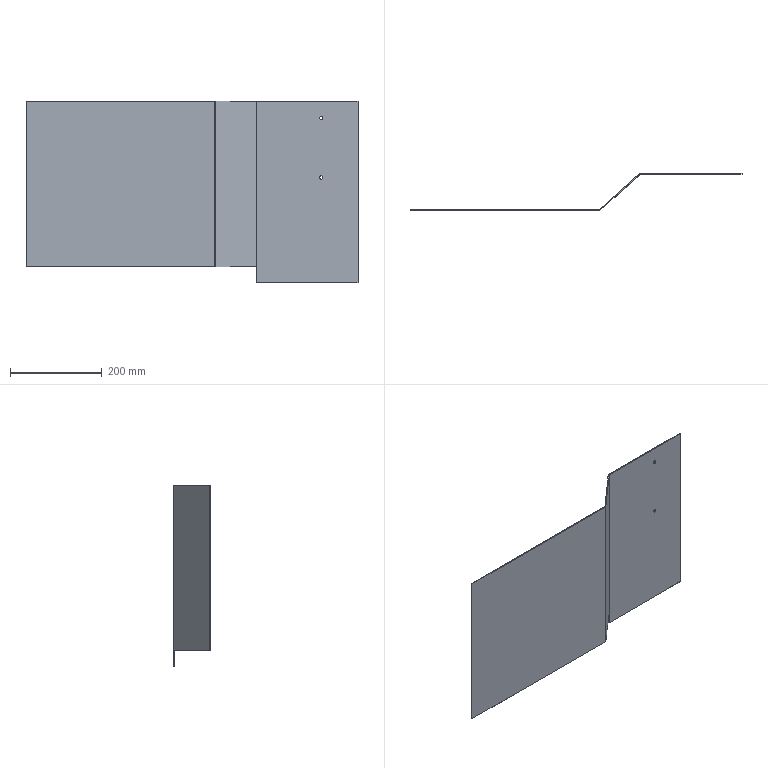Part | STEP file | TX-01-1 | 1 solid | 20 faces | box 724 x 82 x 395 mm | volume 558409 mm3 | plane 12 | cylinder 8 | commonest cylinder face diameters 7 x4 1 x2 5 x2
STEP:
#1=CARTESIAN_POINT('',(182.728,164.713,320.5));
#2=VERTEX_POINT('',#1);
#3=CARTESIAN_POINT('',(182.728,164.713,327.5));
#4=VERTEX_POINT('',#3);
#5=CARTESIAN_POINT('',(182.728,164.713,324.));
#6=DIRECTION('',(0.,1.,0.));
#7=DIRECTION('',(0.,0.,1.));
#8=AXIS2_PLACEMENT_3D('',#5,#6,#7);
#9=CIRCLE('',#8,3.5);
#10=EDGE_CURVE('',#2,#4,#9,.T.);
#11=ORIENTED_EDGE('',*,*,#10,.F.);
#12=CARTESIAN_POINT('',(182.728,166.713,320.5));
#13=VERTEX_POINT('',#12);
#14=CARTESIAN_POINT('',(182.728,156.713,320.5));
#15=DIRECTION('',(0.,1.,0.));
#16=VECTOR('',#15,1000.);
#17=LINE('',#14,#16);
#18=EDGE_CURVE('',#2,#13,#17,.T.);
#19=ORIENTED_EDGE('',*,*,#18,.T.);
#20=CARTESIAN_POINT('',(182.728,166.713,327.5));
#21=VERTEX_POINT('',#20);
#22=CARTESIAN_POINT('',(182.728,166.713,324.));
#23=DIRECTION('',(0.,-1.,0.));
#24=DIRECTION('',(0.,0.,1.));
#25=AXIS2_PLACEMENT_3D('',#22,#23,#24);
#26=CIRCLE('',#25,3.5);
#27=EDGE_CURVE('',#21,#13,#26,.T.);
#28=ORIENTED_EDGE('',*,*,#27,.F.);
#29=CARTESIAN_POINT('',(182.728,156.713,327.5));
#30=DIRECTION('',(0.,1.,0.));
#31=VECTOR('',#30,1000.);
#32=LINE('',#29,#31);
#33=EDGE_CURVE('',#4,#21,#32,.T.);
#34=ORIENTED_EDGE('',*,*,#33,.F.);
#35=EDGE_LOOP('',(#11,#19,#28,#34));
#36=FACE_OUTER_BOUND('',#35,.T.);
#37=CARTESIAN_POINT('',(182.728,156.713,324.));
#38=DIRECTION('',(0.,1.,0.));
#39=DIRECTION('',(0.,0.,1.));
#40=AXIS2_PLACEMENT_3D('',#37,#38,#39);
#41=CYLINDRICAL_SURFACE('',#40,3.5);
#42=ADVANCED_FACE('',(#36),#41,.F.);
#43=CARTESIAN_POINT('',(182.728,164.713,190.5));
#44=VERTEX_POINT('',#43);
#45=CARTESIAN_POINT('',(182.728,164.713,197.5));
#46=VERTEX_POINT('',#45);
#47=CARTESIAN_POINT('',(182.728,164.713,194.));
#48=DIRECTION('',(0.,1.,0.));
#49=DIRECTION('',(0.,0.,1.));
#50=AXIS2_PLACEMENT_3D('',#47,#48,#49);
#51=CIRCLE('',#50,3.5);
#52=EDGE_CURVE('',#44,#46,#51,.T.);
#53=ORIENTED_EDGE('',*,*,#52,.F.);
#54=CARTESIAN_POINT('',(182.728,166.713,190.5));
#55=VERTEX_POINT('',#54);
#56=CARTESIAN_POINT('',(182.728,156.713,190.5));
#57=DIRECTION('',(0.,1.,0.));
#58=VECTOR('',#57,1000.);
#59=LINE('',#56,#58);
#60=EDGE_CURVE('',#44,#55,#59,.T.);
#61=ORIENTED_EDGE('',*,*,#60,.T.);
#62=CARTESIAN_POINT('',(182.728,166.713,197.5));
#63=VERTEX_POINT('',#62);
#64=CARTESIAN_POINT('',(182.728,166.713,194.));
#65=DIRECTION('',(0.,-1.,0.));
#66=DIRECTION('',(0.,0.,1.));
#67=AXIS2_PLACEMENT_3D('',#64,#65,#66);
#68=CIRCLE('',#67,3.5);
#69=EDGE_CURVE('',#63,#55,#68,.T.);
#70=ORIENTED_EDGE('',*,*,#69,.F.);
#71=CARTESIAN_POINT('',(182.728,156.713,197.5));
#72=DIRECTION('',(0.,1.,0.));
#73=VECTOR('',#72,1000.);
#74=LINE('',#71,#73);
#75=EDGE_CURVE('',#46,#63,#74,.T.);
#76=ORIENTED_EDGE('',*,*,#75,.F.);
#77=EDGE_LOOP('',(#53,#61,#70,#76));
#78=FACE_OUTER_BOUND('',#77,.T.);
#79=CARTESIAN_POINT('',(182.728,156.713,194.));
#80=DIRECTION('',(0.,1.,0.));
#81=DIRECTION('',(0.,0.,1.));
#82=AXIS2_PLACEMENT_3D('',#79,#80,#81);
#83=CYLINDRICAL_SURFACE('',#82,3.5);
#84=ADVANCED_FACE('',(#78),#83,.F.);
#85=CARTESIAN_POINT('',(-461.272,86.713,360.));
#86=VERTEX_POINT('',#85);
#87=CARTESIAN_POINT('',(-49.223,86.713,360.));
#88=VERTEX_POINT('',#87);
#89=CARTESIAN_POINT('',(-48.272,86.713,360.));
#90=DIRECTION('',(1.,0.,0.));
#91=VECTOR('',#90,1000.);
#92=LINE('',#89,#91);
#93=EDGE_CURVE('',#86,#88,#92,.T.);
#94=ORIENTED_EDGE('',*,*,#93,.T.);
#95=CARTESIAN_POINT('',(-49.223,86.713,0.));
#96=VERTEX_POINT('',#95);
#97=CARTESIAN_POINT('',(-49.223,86.713,360.));
#98=DIRECTION('',(0.,0.,-1.));
#99=VECTOR('',#98,1000.);
#100=LINE('',#97,#99);
#101=EDGE_CURVE('',#88,#96,#100,.T.);
#102=ORIENTED_EDGE('',*,*,#101,.T.);
#103=CARTESIAN_POINT('',(-461.272,86.713,0.));
#104=VERTEX_POINT('',#103);
#105=CARTESIAN_POINT('',(-48.272,86.713,0.));
#106=DIRECTION('',(-1.,0.,0.));
#107=VECTOR('',#106,1000.);
#108=LINE('',#105,#107);
#109=EDGE_CURVE('',#96,#104,#108,.T.);
#110=ORIENTED_EDGE('',*,*,#109,.T.);
#111=CARTESIAN_POINT('',(-461.272,86.713,360.));
#112=DIRECTION('',(0.,0.,1.));
#113=VECTOR('',#112,1000.);
#114=LINE('',#111,#113);
#115=EDGE_CURVE('',#104,#86,#114,.T.);
#116=ORIENTED_EDGE('',*,*,#115,.T.);
#117=EDGE_LOOP('',(#94,#102,#110,#116));
#118=FACE_OUTER_BOUND('',#117,.T.);
#119=CARTESIAN_POINT('',(-48.272,86.713,360.));
#120=DIRECTION('',(0.,1.,0.));
#121=DIRECTION('',(-1.,0.,0.));
#122=AXIS2_PLACEMENT_3D('',#119,#120,#121);
#123=PLANE('',#122);
#124=ADVANCED_FACE('',(#118),#123,.T.);
#125=ORIENTED_EDGE('',*,*,#101,.F.);
#126=CARTESIAN_POINT('',(-48.891,86.839,360.));
#127=VERTEX_POINT('',#126);
#128=CARTESIAN_POINT('',(-49.223,87.213,360.));
#129=DIRECTION('',(0.,0.,-1.));
#130=DIRECTION('',(-1.,0.,0.));
#131=AXIS2_PLACEMENT_3D('',#128,#129,#130);
#132=CIRCLE('',#131,0.5);
#133=EDGE_CURVE('',#127,#88,#132,.T.);
#134=ORIENTED_EDGE('',*,*,#133,.F.);
#135=CARTESIAN_POINT('',(-48.891,86.839,0.));
#136=VERTEX_POINT('',#135);
#137=CARTESIAN_POINT('',(-48.891,86.839,360.));
#138=DIRECTION('',(0.,0.,1.));
#139=VECTOR('',#138,1000.);
#140=LINE('',#137,#139);
#141=EDGE_CURVE('',#136,#127,#140,.T.);
#142=ORIENTED_EDGE('',*,*,#141,.F.);
#143=CARTESIAN_POINT('',(-49.223,87.213,0.));
#144=DIRECTION('',(0.,0.,1.));
#145=DIRECTION('',(-1.,0.,0.));
#146=AXIS2_PLACEMENT_3D('',#143,#144,#145);
#147=CIRCLE('',#146,0.5);
#148=EDGE_CURVE('',#96,#136,#147,.T.);
#149=ORIENTED_EDGE('',*,*,#148,.F.);
#150=EDGE_LOOP('',(#125,#134,#142,#149));
#151=FACE_OUTER_BOUND('',#150,.T.);
#152=CARTESIAN_POINT('',(-49.223,87.213,360.));
#153=DIRECTION('',(0.,0.,-1.));
#154=DIRECTION('',(-1.,0.,0.));
#155=AXIS2_PLACEMENT_3D('',#152,#153,#154);
#156=CYLINDRICAL_SURFACE('',#155,0.5);
#157=ADVANCED_FACE('',(#151),#156,.F.);
#158=ORIENTED_EDGE('',*,*,#93,.F.);
#159=CARTESIAN_POINT('',(-461.272,84.713,360.));
#160=VERTEX_POINT('',#159);
#161=CARTESIAN_POINT('',(-461.272,86.839,360.));
#162=DIRECTION('',(0.,-1.,0.));
#163=VECTOR('',#162,1000.);
#164=LINE('',#161,#163);
#165=EDGE_CURVE('',#86,#160,#164,.T.);
#166=ORIENTED_EDGE('',*,*,#165,.T.);
#167=CARTESIAN_POINT('',(-49.223,84.713,360.));
#168=VERTEX_POINT('',#167);
#169=CARTESIAN_POINT('',(-48.891,84.713,360.));
#170=DIRECTION('',(1.,0.,0.));
#171=VECTOR('',#170,1000.);
#172=LINE('',#169,#171);
#173=EDGE_CURVE('',#160,#168,#172,.T.);
#174=ORIENTED_EDGE('',*,*,#173,.T.);
#175=CARTESIAN_POINT('',(-47.562,85.344,360.));
#176=VERTEX_POINT('',#175);
#177=CARTESIAN_POINT('',(-49.223,87.213,360.));
#178=DIRECTION('',(0.,0.,1.));
#179=DIRECTION('',(-1.,0.,0.));
#180=AXIS2_PLACEMENT_3D('',#177,#178,#179);
#181=CIRCLE('',#180,2.5);
#182=EDGE_CURVE('',#168,#176,#181,.T.);
#183=ORIENTED_EDGE('',*,*,#182,.T.);
#184=CARTESIAN_POINT('',(41.585,164.587,360.));
#185=VERTEX_POINT('',#184);
#186=CARTESIAN_POINT('',(-47.562,85.344,360.));
#187=DIRECTION('',(0.7474,0.6644,0.));
#188=VECTOR('',#187,1000.);
#189=LINE('',#186,#188);
#190=EDGE_CURVE('',#176,#185,#189,.T.);
#191=ORIENTED_EDGE('',*,*,#190,.T.);
#192=CARTESIAN_POINT('',(41.918,164.713,360.));
#193=VERTEX_POINT('',#192);
#194=CARTESIAN_POINT('',(41.918,164.213,360.));
#195=DIRECTION('',(0.,0.,-1.));
#196=DIRECTION('',(-1.,0.,0.));
#197=AXIS2_PLACEMENT_3D('',#194,#195,#196);
#198=CIRCLE('',#197,0.5);
#199=EDGE_CURVE('',#185,#193,#198,.T.);
#200=ORIENTED_EDGE('',*,*,#199,.T.);
#201=CARTESIAN_POINT('',(262.728,164.713,360.));
#202=VERTEX_POINT('',#201);
#203=CARTESIAN_POINT('',(41.918,164.713,360.));
#204=DIRECTION('',(1.,0.,0.));
#205=VECTOR('',#204,1000.);
#206=LINE('',#203,#205);
#207=EDGE_CURVE('',#193,#202,#206,.T.);
#208=ORIENTED_EDGE('',*,*,#207,.T.);
#209=CARTESIAN_POINT('',(262.728,166.713,360.));
#210=VERTEX_POINT('',#209);
#211=CARTESIAN_POINT('',(262.728,164.213,360.));
#212=DIRECTION('',(0.,1.,0.));
#213=VECTOR('',#212,1000.);
#214=LINE('',#211,#213);
#215=EDGE_CURVE('',#202,#210,#214,.T.);
#216=ORIENTED_EDGE('',*,*,#215,.T.);
#217=CARTESIAN_POINT('',(41.918,166.713,360.));
#218=VERTEX_POINT('',#217);
#219=CARTESIAN_POINT('',(41.728,166.713,360.));
#220=DIRECTION('',(1.,0.,0.));
#221=VECTOR('',#220,1000.);
#222=LINE('',#219,#221);
#223=EDGE_CURVE('',#218,#210,#222,.T.);
#224=ORIENTED_EDGE('',*,*,#223,.F.);
#225=CARTESIAN_POINT('',(40.257,166.081,360.));
#226=VERTEX_POINT('',#225);
#227=CARTESIAN_POINT('',(41.918,164.213,360.));
#228=DIRECTION('',(0.,0.,-1.));
#229=DIRECTION('',(-1.,0.,0.));
#230=AXIS2_PLACEMENT_3D('',#227,#228,#229);
#231=CIRCLE('',#230,2.5);
#232=EDGE_CURVE('',#226,#218,#231,.T.);
#233=ORIENTED_EDGE('',*,*,#232,.F.);
#234=CARTESIAN_POINT('',(40.399,166.208,360.));
#235=DIRECTION('',(0.7474,0.6644,0.));
#236=VECTOR('',#235,1000.);
#237=LINE('',#234,#236);
#238=EDGE_CURVE('',#127,#226,#237,.T.);
#239=ORIENTED_EDGE('',*,*,#238,.F.);
#240=ORIENTED_EDGE('',*,*,#133,.T.);
#241=EDGE_LOOP('',(#158,#166,#174,#183,#191,#200,#208,#216,#224,#233,#239,#240));
#242=FACE_OUTER_BOUND('',#241,.T.);
#243=CARTESIAN_POINT('',(-48.891,86.839,360.));
#244=DIRECTION('',(0.,0.,1.));
#245=DIRECTION('',(1.,0.,0.));
#246=AXIS2_PLACEMENT_3D('',#243,#244,#245);
#247=PLANE('',#246);
#248=ADVANCED_FACE('',(#242),#247,.T.);
#249=ORIENTED_EDGE('',*,*,#165,.F.);
#250=ORIENTED_EDGE('',*,*,#115,.F.);
#251=CARTESIAN_POINT('',(-461.272,84.713,0.));
#252=VERTEX_POINT('',#251);
#253=CARTESIAN_POINT('',(-461.272,84.713,0.));
#254=DIRECTION('',(0.,-1.,0.));
#255=VECTOR('',#254,1000.);
#256=LINE('',#253,#255);
#257=EDGE_CURVE('',#104,#252,#256,.T.);
#258=ORIENTED_EDGE('',*,*,#257,.T.);
#259=CARTESIAN_POINT('',(-461.272,84.713,360.));
#260=DIRECTION('',(0.,0.,1.));
#261=VECTOR('',#260,1000.);
#262=LINE('',#259,#261);
#263=EDGE_CURVE('',#252,#160,#262,.T.);
#264=ORIENTED_EDGE('',*,*,#263,.T.);
#265=EDGE_LOOP('',(#249,#250,#258,#264));
#266=FACE_OUTER_BOUND('',#265,.T.);
#267=CARTESIAN_POINT('',(-461.272,84.713,360.));
#268=DIRECTION('',(-1.,0.,0.));
#269=DIRECTION('',(0.,0.,1.));
#270=AXIS2_PLACEMENT_3D('',#267,#268,#269);
#271=PLANE('',#270);
#272=ADVANCED_FACE('',(#266),#271,.T.);
#273=ORIENTED_EDGE('',*,*,#109,.F.);
#274=ORIENTED_EDGE('',*,*,#148,.T.);
#275=CARTESIAN_POINT('',(40.257,166.081,0.));
#276=VERTEX_POINT('',#275);
#277=CARTESIAN_POINT('',(40.399,166.208,0.));
#278=DIRECTION('',(-0.7474,-0.6644,0.));
#279=VECTOR('',#278,1000.);
#280=LINE('',#277,#279);
#281=EDGE_CURVE('',#276,#136,#280,.T.);
#282=ORIENTED_EDGE('',*,*,#281,.F.);
#283=CARTESIAN_POINT('',(41.918,166.713,0.));
#284=VERTEX_POINT('',#283);
#285=CARTESIAN_POINT('',(41.918,164.213,0.));
#286=DIRECTION('',(0.,0.,1.));
#287=DIRECTION('',(-1.,0.,0.));
#288=AXIS2_PLACEMENT_3D('',#285,#286,#287);
#289=CIRCLE('',#288,2.5);
#290=EDGE_CURVE('',#284,#276,#289,.T.);
#291=ORIENTED_EDGE('',*,*,#290,.F.);
#292=CARTESIAN_POINT('',(41.918,164.713,0.));
#293=VERTEX_POINT('',#292);
#294=CARTESIAN_POINT('',(41.918,164.713,0.));
#295=DIRECTION('',(0.,-1.,0.));
#296=VECTOR('',#295,1000.);
#297=LINE('',#294,#296);
#298=EDGE_CURVE('',#284,#293,#297,.T.);
#299=ORIENTED_EDGE('',*,*,#298,.T.);
#300=CARTESIAN_POINT('',(41.585,164.587,0.));
#301=VERTEX_POINT('',#300);
#302=CARTESIAN_POINT('',(41.918,164.213,0.));
#303=DIRECTION('',(0.,0.,1.));
#304=DIRECTION('',(-1.,0.,0.));
#305=AXIS2_PLACEMENT_3D('',#302,#303,#304);
#306=CIRCLE('',#305,0.5);
#307=EDGE_CURVE('',#293,#301,#306,.T.);
#308=ORIENTED_EDGE('',*,*,#307,.T.);
#309=CARTESIAN_POINT('',(-47.562,85.344,0.));
#310=VERTEX_POINT('',#309);
#311=CARTESIAN_POINT('',(41.585,164.587,0.));
#312=DIRECTION('',(-0.7474,-0.6644,0.));
#313=VECTOR('',#312,1000.);
#314=LINE('',#311,#313);
#315=EDGE_CURVE('',#301,#310,#314,.T.);
#316=ORIENTED_EDGE('',*,*,#315,.T.);
#317=CARTESIAN_POINT('',(-49.223,84.713,0.));
#318=VERTEX_POINT('',#317);
#319=CARTESIAN_POINT('',(-49.223,87.213,0.));
#320=DIRECTION('',(0.,0.,-1.));
#321=DIRECTION('',(-1.,0.,0.));
#322=AXIS2_PLACEMENT_3D('',#319,#320,#321);
#323=CIRCLE('',#322,2.5);
#324=EDGE_CURVE('',#310,#318,#323,.T.);
#325=ORIENTED_EDGE('',*,*,#324,.T.);
#326=CARTESIAN_POINT('',(41.918,84.713,0.));
#327=DIRECTION('',(1.,0.,0.));
#328=VECTOR('',#327,1000.);
#329=LINE('',#326,#328);
#330=EDGE_CURVE('',#252,#318,#329,.T.);
#331=ORIENTED_EDGE('',*,*,#330,.F.);
#332=ORIENTED_EDGE('',*,*,#257,.F.);
#333=EDGE_LOOP('',(#273,#274,#282,#291,#299,#308,#316,#325,#331,#332));
#334=FACE_OUTER_BOUND('',#333,.T.);
#335=CARTESIAN_POINT('',(41.918,164.213,0.));
#336=DIRECTION('',(0.,0.,1.));
#337=DIRECTION('',(1.,0.,0.));
#338=AXIS2_PLACEMENT_3D('',#335,#336,#337);
#339=PLANE('',#338);
#340=ADVANCED_FACE('',(#334),#339,.F.);
#341=ORIENTED_EDGE('',*,*,#238,.T.);
#342=CARTESIAN_POINT('',(40.257,166.081,360.));
#343=DIRECTION('',(0.,0.,-1.));
#344=VECTOR('',#343,1000.);
#345=LINE('',#342,#344);
#346=EDGE_CURVE('',#226,#276,#345,.T.);
#347=ORIENTED_EDGE('',*,*,#346,.T.);
#348=ORIENTED_EDGE('',*,*,#281,.T.);
#349=ORIENTED_EDGE('',*,*,#141,.T.);
#350=EDGE_LOOP('',(#341,#347,#348,#349));
#351=FACE_OUTER_BOUND('',#350,.T.);
#352=CARTESIAN_POINT('',(40.399,166.208,360.));
#353=DIRECTION('',(-0.6644,0.7474,0.));
#354=DIRECTION('',(-0.7474,-0.6644,0.));
#355=AXIS2_PLACEMENT_3D('',#352,#353,#354);
#356=PLANE('',#355);
#357=ADVANCED_FACE('',(#351),#356,.T.);
#358=CARTESIAN_POINT('',(-49.223,84.713,360.));
#359=DIRECTION('',(0.,0.,-1.));
#360=VECTOR('',#359,1000.);
#361=LINE('',#358,#360);
#362=EDGE_CURVE('',#168,#318,#361,.T.);
#363=ORIENTED_EDGE('',*,*,#362,.F.);
#364=ORIENTED_EDGE('',*,*,#173,.F.);
#365=ORIENTED_EDGE('',*,*,#263,.F.);
#366=ORIENTED_EDGE('',*,*,#330,.T.);
#367=EDGE_LOOP('',(#363,#364,#365,#366));
#368=FACE_OUTER_BOUND('',#367,.T.);
#369=CARTESIAN_POINT('',(-48.272,84.713,360.));
#370=DIRECTION('',(0.,1.,0.));
#371=DIRECTION('',(-1.,0.,0.));
#372=AXIS2_PLACEMENT_3D('',#369,#370,#371);
#373=PLANE('',#372);
#374=ADVANCED_FACE('',(#368),#373,.F.);
#375=ORIENTED_EDGE('',*,*,#232,.T.);
#376=CARTESIAN_POINT('',(41.918,166.713,360.));
#377=DIRECTION('',(0.,0.,-1.));
#378=VECTOR('',#377,1000.);
#379=LINE('',#376,#378);
#380=EDGE_CURVE('',#218,#284,#379,.T.);
#381=ORIENTED_EDGE('',*,*,#380,.T.);
#382=ORIENTED_EDGE('',*,*,#290,.T.);
#383=ORIENTED_EDGE('',*,*,#346,.F.);
#384=EDGE_LOOP('',(#375,#381,#382,#383));
#385=FACE_OUTER_BOUND('',#384,.T.);
#386=CARTESIAN_POINT('',(41.918,164.213,360.));
#387=DIRECTION('',(0.,0.,-1.));
#388=DIRECTION('',(-1.,0.,0.));
#389=AXIS2_PLACEMENT_3D('',#386,#387,#388);
#390=CYLINDRICAL_SURFACE('',#389,2.5);
#391=ADVANCED_FACE('',(#385),#390,.T.);
#392=ORIENTED_EDGE('',*,*,#182,.F.);
#393=ORIENTED_EDGE('',*,*,#362,.T.);
#394=ORIENTED_EDGE('',*,*,#324,.F.);
#395=CARTESIAN_POINT('',(-47.562,85.344,360.));
#396=DIRECTION('',(0.,0.,1.));
#397=VECTOR('',#396,1000.);
#398=LINE('',#395,#397);
#399=EDGE_CURVE('',#310,#176,#398,.T.);
#400=ORIENTED_EDGE('',*,*,#399,.T.);
#401=EDGE_LOOP('',(#392,#393,#394,#400));
#402=FACE_OUTER_BOUND('',#401,.T.);
#403=CARTESIAN_POINT('',(-49.223,87.213,360.));
#404=DIRECTION('',(0.,0.,-1.));
#405=DIRECTION('',(-1.,0.,0.));
#406=AXIS2_PLACEMENT_3D('',#403,#404,#405);
#407=CYLINDRICAL_SURFACE('',#406,2.5);
#408=ADVANCED_FACE('',(#402),#407,.T.);
#409=ORIENTED_EDGE('',*,*,#380,.F.);
#410=ORIENTED_EDGE('',*,*,#223,.T.);
#411=CARTESIAN_POINT('',(262.728,166.713,-35.));
#412=VERTEX_POINT('',#411);
#413=CARTESIAN_POINT('',(262.728,166.713,360.));
#414=DIRECTION('',(0.,0.,-1.));
#415=VECTOR('',#414,1000.);
#416=LINE('',#413,#415);
#417=EDGE_CURVE('',#210,#412,#416,.T.);
#418=ORIENTED_EDGE('',*,*,#417,.T.);
#419=CARTESIAN_POINT('',(41.918,166.713,-35.));
#420=VERTEX_POINT('',#419);
#421=CARTESIAN_POINT('',(41.728,166.713,-35.));
#422=DIRECTION('',(-1.,0.,0.));
#423=VECTOR('',#422,1000.);
#424=LINE('',#421,#423);
#425=EDGE_CURVE('',#412,#420,#424,.T.);
#426=ORIENTED_EDGE('',*,*,#425,.T.);
#427=CARTESIAN_POINT('',(41.918,166.713,360.));
#428=DIRECTION('',(0.,0.,1.));
#429=VECTOR('',#428,1000.);
#430=LINE('',#427,#429);
#431=EDGE_CURVE('',#420,#284,#430,.T.);
#432=ORIENTED_EDGE('',*,*,#431,.T.);
#433=EDGE_LOOP('',(#409,#410,#418,#426,#432));
#434=FACE_OUTER_BOUND('',#433,.T.);
#435=ORIENTED_EDGE('',*,*,#27,.T.);
#436=CARTESIAN_POINT('',(182.728,166.713,324.));
#437=DIRECTION('',(0.,-1.,0.));
#438=DIRECTION('',(0.,0.,1.));
#439=AXIS2_PLACEMENT_3D('',#436,#437,#438);
#440=CIRCLE('',#439,3.5);
#441=EDGE_CURVE('',#13,#21,#440,.T.);
#442=ORIENTED_EDGE('',*,*,#441,.T.);
#443=EDGE_LOOP('',(#435,#442));
#444=FACE_BOUND('',#443,.T.);
#445=ORIENTED_EDGE('',*,*,#69,.T.);
#446=CARTESIAN_POINT('',(182.728,166.713,194.));
#447=DIRECTION('',(0.,-1.,0.));
#448=DIRECTION('',(0.,0.,1.));
#449=AXIS2_PLACEMENT_3D('',#446,#447,#448);
#450=CIRCLE('',#449,3.5);
#451=EDGE_CURVE('',#55,#63,#450,.T.);
#452=ORIENTED_EDGE('',*,*,#451,.T.);
#453=EDGE_LOOP('',(#445,#452));
#454=FACE_BOUND('',#453,.T.);
#455=CARTESIAN_POINT('',(41.728,166.713,360.));
#456=DIRECTION('',(0.,1.,0.));
#457=DIRECTION('',(0.,0.,1.));
#458=AXIS2_PLACEMENT_3D('',#455,#456,#457);
#459=PLANE('',#458);
#460=ADVANCED_FACE('',(#434,#444,#454),#459,.T.);
#461=CARTESIAN_POINT('',(41.585,164.587,360.));
#462=DIRECTION('',(0.,0.,-1.));
#463=VECTOR('',#462,1000.);
#464=LINE('',#461,#463);
#465=EDGE_CURVE('',#185,#301,#464,.T.);
#466=ORIENTED_EDGE('',*,*,#465,.F.);
#467=ORIENTED_EDGE('',*,*,#190,.F.);
#468=ORIENTED_EDGE('',*,*,#399,.F.);
#469=ORIENTED_EDGE('',*,*,#315,.F.);
#470=EDGE_LOOP('',(#466,#467,#468,#469));
#471=FACE_OUTER_BOUND('',#470,.T.);
#472=CARTESIAN_POINT('',(41.728,164.713,360.));
#473=DIRECTION('',(-0.6644,0.7474,0.));
#474=DIRECTION('',(-0.7474,-0.6644,0.));
#475=AXIS2_PLACEMENT_3D('',#472,#473,#474);
#476=PLANE('',#475);
#477=ADVANCED_FACE('',(#471),#476,.F.);
#478=ORIENTED_EDGE('',*,*,#431,.F.);
#479=CARTESIAN_POINT('',(41.918,164.713,-35.));
#480=VERTEX_POINT('',#479);
#481=CARTESIAN_POINT('',(41.918,166.713,-35.));
#482=DIRECTION('',(0.,1.,0.));
#483=VECTOR('',#482,1000.);
#484=LINE('',#481,#483);
#485=EDGE_CURVE('',#480,#420,#484,.T.);
#486=ORIENTED_EDGE('',*,*,#485,.F.);
#487=CARTESIAN_POINT('',(41.918,164.713,-35.));
#488=DIRECTION('',(0.,0.,-1.));
#489=VECTOR('',#488,1000.);
#490=LINE('',#487,#489);
#491=EDGE_CURVE('',#293,#480,#490,.T.);
#492=ORIENTED_EDGE('',*,*,#491,.F.);
#493=ORIENTED_EDGE('',*,*,#298,.F.);
#494=EDGE_LOOP('',(#478,#486,#492,#493));
#495=FACE_OUTER_BOUND('',#494,.T.);
#496=CARTESIAN_POINT('',(41.918,166.713,-35.));
#497=DIRECTION('',(1.,0.,0.));
#498=DIRECTION('',(0.,0.,-1.));
#499=AXIS2_PLACEMENT_3D('',#496,#497,#498);
#500=PLANE('',#499);
#501=ADVANCED_FACE('',(#495),#500,.F.);
#502=ORIENTED_EDGE('',*,*,#485,.T.);
#503=ORIENTED_EDGE('',*,*,#425,.F.);
#504=CARTESIAN_POINT('',(262.728,164.713,-35.));
#505=VERTEX_POINT('',#504);
#506=CARTESIAN_POINT('',(262.728,0.,-35.));
#507=DIRECTION('',(0.,-1.,0.));
#508=VECTOR('',#507,1000.);
#509=LINE('',#506,#508);
#510=EDGE_CURVE('',#412,#505,#509,.T.);
#511=ORIENTED_EDGE('',*,*,#510,.T.);
#512=CARTESIAN_POINT('',(0.,164.713,-35.));
#513=DIRECTION('',(-1.,0.,0.));
#514=VECTOR('',#513,1000.);
#515=LINE('',#512,#514);
#516=EDGE_CURVE('',#505,#480,#515,.T.);
#517=ORIENTED_EDGE('',*,*,#516,.T.);
#518=EDGE_LOOP('',(#502,#503,#511,#517));
#519=FACE_OUTER_BOUND('',#518,.T.);
#520=CARTESIAN_POINT('',(0.,0.,-35.));
#521=DIRECTION('',(0.,0.,-1.));
#522=DIRECTION('',(-1.,0.,0.));
#523=AXIS2_PLACEMENT_3D('',#520,#521,#522);
#524=PLANE('',#523);
#525=ADVANCED_FACE('',(#519),#524,.T.);
#526=ORIENTED_EDGE('',*,*,#417,.F.);
#527=ORIENTED_EDGE('',*,*,#215,.F.);
#528=CARTESIAN_POINT('',(262.728,164.713,360.));
#529=DIRECTION('',(0.,0.,-1.));
#530=VECTOR('',#529,1000.);
#531=LINE('',#528,#530);
#532=EDGE_CURVE('',#202,#505,#531,.T.);
#533=ORIENTED_EDGE('',*,*,#532,.T.);
#534=ORIENTED_EDGE('',*,*,#510,.F.);
#535=EDGE_LOOP('',(#526,#527,#533,#534));
#536=FACE_OUTER_BOUND('',#535,.T.);
#537=CARTESIAN_POINT('',(262.728,166.713,360.));
#538=DIRECTION('',(1.,0.,0.));
#539=DIRECTION('',(0.,0.,-1.));
#540=AXIS2_PLACEMENT_3D('',#537,#538,#539);
#541=PLANE('',#540);
#542=ADVANCED_FACE('',(#536),#541,.T.);
#543=ORIENTED_EDGE('',*,*,#18,.F.);
#544=CARTESIAN_POINT('',(182.728,164.713,324.));
#545=DIRECTION('',(0.,1.,0.));
#546=DIRECTION('',(0.,0.,1.));
#547=AXIS2_PLACEMENT_3D('',#544,#545,#546);
#548=CIRCLE('',#547,3.5);
#549=EDGE_CURVE('',#4,#2,#548,.T.);
#550=ORIENTED_EDGE('',*,*,#549,.F.);
#551=ORIENTED_EDGE('',*,*,#33,.T.);
#552=ORIENTED_EDGE('',*,*,#441,.F.);
#553=EDGE_LOOP('',(#543,#550,#551,#552));
#554=FACE_OUTER_BOUND('',#553,.T.);
#555=CARTESIAN_POINT('',(182.728,156.713,324.));
#556=DIRECTION('',(0.,1.,0.));
#557=DIRECTION('',(0.,0.,1.));
#558=AXIS2_PLACEMENT_3D('',#555,#556,#557);
#559=CYLINDRICAL_SURFACE('',#558,3.5);
#560=ADVANCED_FACE('',(#554),#559,.F.);
#561=ORIENTED_EDGE('',*,*,#60,.F.);
#562=CARTESIAN_POINT('',(182.728,164.713,194.));
#563=DIRECTION('',(0.,1.,0.));
#564=DIRECTION('',(0.,0.,1.));
#565=AXIS2_PLACEMENT_3D('',#562,#563,#564);
#566=CIRCLE('',#565,3.5);
#567=EDGE_CURVE('',#46,#44,#566,.T.);
#568=ORIENTED_EDGE('',*,*,#567,.F.);
#569=ORIENTED_EDGE('',*,*,#75,.T.);
#570=ORIENTED_EDGE('',*,*,#451,.F.);
#571=EDGE_LOOP('',(#561,#568,#569,#570));
#572=FACE_OUTER_BOUND('',#571,.T.);
#573=CARTESIAN_POINT('',(182.728,156.713,194.));
#574=DIRECTION('',(0.,1.,0.));
#575=DIRECTION('',(0.,0.,1.));
#576=AXIS2_PLACEMENT_3D('',#573,#574,#575);
#577=CYLINDRICAL_SURFACE('',#576,3.5);
#578=ADVANCED_FACE('',(#572),#577,.F.);
#579=CARTESIAN_POINT('',(41.918,164.713,360.));
#580=DIRECTION('',(0.,0.,-1.));
#581=VECTOR('',#580,1000.);
#582=LINE('',#579,#581);
#583=EDGE_CURVE('',#193,#293,#582,.T.);
#584=ORIENTED_EDGE('',*,*,#583,.F.);
#585=ORIENTED_EDGE('',*,*,#199,.F.);
#586=ORIENTED_EDGE('',*,*,#465,.T.);
#587=ORIENTED_EDGE('',*,*,#307,.F.);
#588=EDGE_LOOP('',(#584,#585,#586,#587));
#589=FACE_OUTER_BOUND('',#588,.T.);
#590=CARTESIAN_POINT('',(41.918,164.213,360.));
#591=DIRECTION('',(0.,0.,-1.));
#592=DIRECTION('',(-1.,0.,0.));
#593=AXIS2_PLACEMENT_3D('',#590,#591,#592);
#594=CYLINDRICAL_SURFACE('',#593,0.5);
#595=ADVANCED_FACE('',(#589),#594,.F.);
#596=ORIENTED_EDGE('',*,*,#491,.T.);
#597=ORIENTED_EDGE('',*,*,#516,.F.);
#598=ORIENTED_EDGE('',*,*,#532,.F.);
#599=ORIENTED_EDGE('',*,*,#207,.F.);
#600=ORIENTED_EDGE('',*,*,#583,.T.);
#601=EDGE_LOOP('',(#596,#597,#598,#599,#600));
#602=FACE_OUTER_BOUND('',#601,.T.);
#603=ORIENTED_EDGE('',*,*,#549,.T.);
#604=ORIENTED_EDGE('',*,*,#10,.T.);
#605=EDGE_LOOP('',(#603,#604));
#606=FACE_BOUND('',#605,.T.);
#607=ORIENTED_EDGE('',*,*,#567,.T.);
#608=ORIENTED_EDGE('',*,*,#52,.T.);
#609=EDGE_LOOP('',(#607,#608));
#610=FACE_BOUND('',#609,.T.);
#611=CARTESIAN_POINT('',(41.728,164.713,360.));
#612=DIRECTION('',(0.,1.,0.));
#613=DIRECTION('',(0.,0.,1.));
#614=AXIS2_PLACEMENT_3D('',#611,#612,#613);
#615=PLANE('',#614);
#616=ADVANCED_FACE('',(#602,#606,#610),#615,.F.);
#617=CLOSED_SHELL('',(#42,#84,#124,#157,#248,#272,#340,#357,#374,#391,#408,#460,#477,#501,#525,#542,#560,#578,#595,#616));
#618=MANIFOLD_SOLID_BREP('',#617);
#619=CARTESIAN_POINT('',(0.,0.,0.));
#620=DIRECTION('',(0.,0.,1.));
#621=DIRECTION('',(1.,0.,0.));
#622=AXIS2_PLACEMENT_3D('',#619,#620,#621);
#623=(LENGTH_UNIT()NAMED_UNIT(*)SI_UNIT(.MILLI.,.METRE.));
#624=UNCERTAINTY_MEASURE_WITH_UNIT(LENGTH_MEASURE(0.00001),#623,'','');
#625=(NAMED_UNIT(*)PLANE_ANGLE_UNIT()SI_UNIT($,.RADIAN.));
#626=(NAMED_UNIT(*)SI_UNIT($,.STERADIAN.)SOLID_ANGLE_UNIT());
#627=(GEOMETRIC_REPRESENTATION_CONTEXT(3)GLOBAL_UNCERTAINTY_ASSIGNED_CONTEXT((#624))GLOBAL_UNIT_ASSIGNED_CONTEXT((#623,#625,#626))REPRESENTATION_CONTEXT('',''));
#628=ADVANCED_BREP_SHAPE_REPRESENTATION('',(#618,#622),#627);